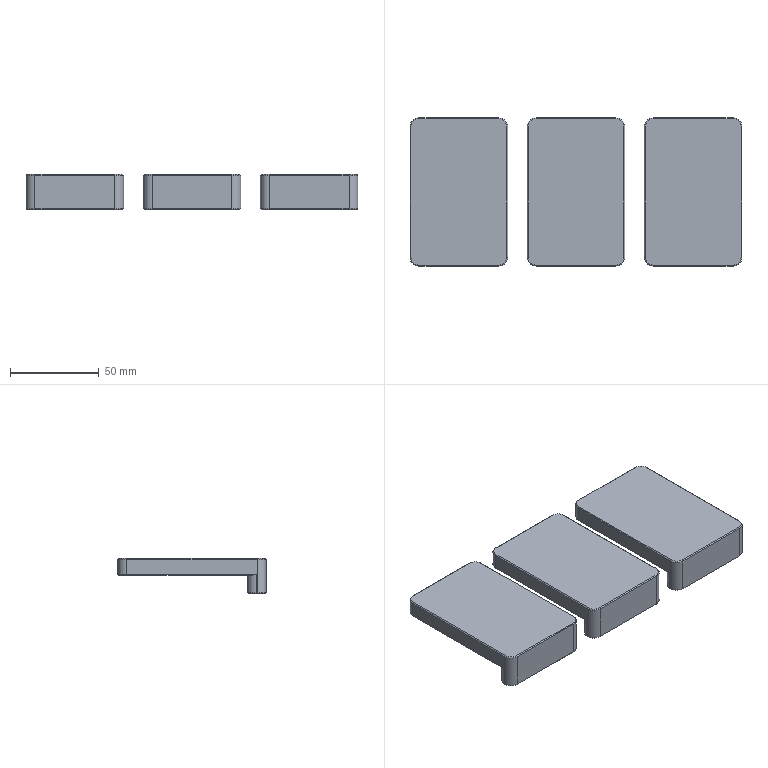NC program | NX | posted with a generic post | part box 187 x 83.5 x 20 mm
Lines 1 to 20 of 5666:
N10 G17 G21 G94 G90
(FLOOR_WALL , TOOL : D80)
N12 T19 M6
N14 G54
N16 G17 G0 G90 X-138.5 Y43.747 S6500 M3
N18 G43 Z30. H19
N20 Z3.
N22 G94 G1 Z0. F1500.
N24 X-135.5
N26 X135.5
N28 Y-11.75
N30 X-135.5
N32 X-138.5
N34 Z3.
N36 G0 Z30.
N38 M5